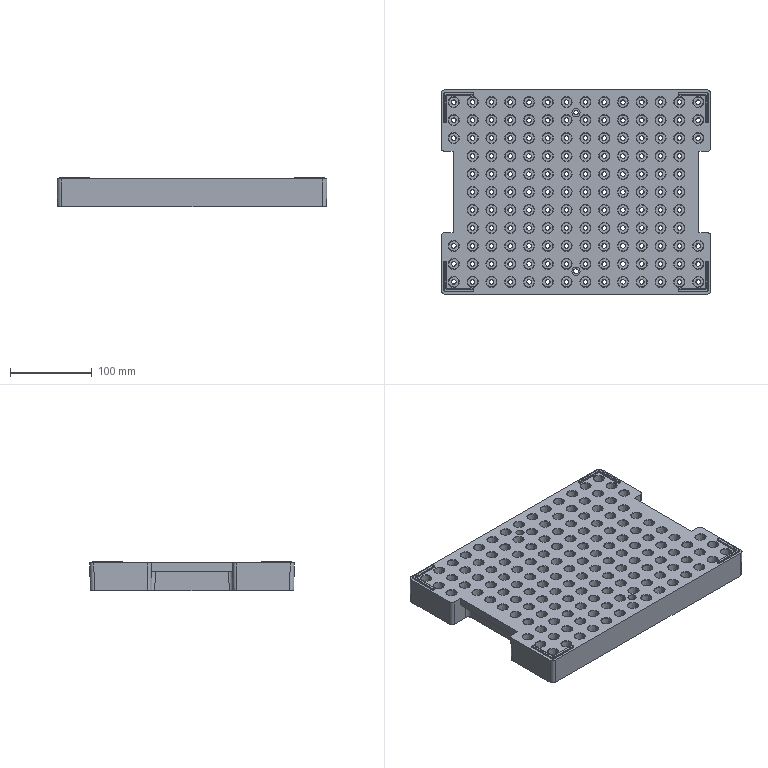Part | SolidWorks | features BaseBody 1 | 1 solid | 3145 faces | volume 715592 mm3 | plane 1589 | cone 1443 | cylinder 89 | spline 24 | commonest cylinder face diameters 1 x28 2 x20 10 x16 14 x8 6 x6 4 x5